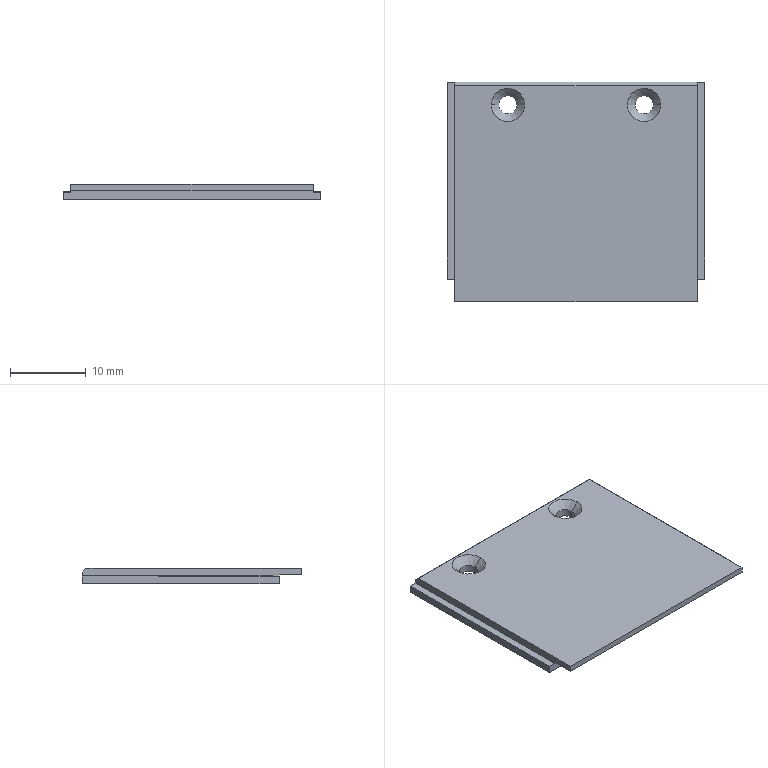Part | STEP file | ASND-0110-OPT-CO40-X-V1.0 upper cover plate | 1 solid | 21 faces | box 34 x 29 x 2 mm | volume 1761 mm3 | plane 13 | cone 4 | cylinder 4 | commonest cylinder face diameters 2.4 x4